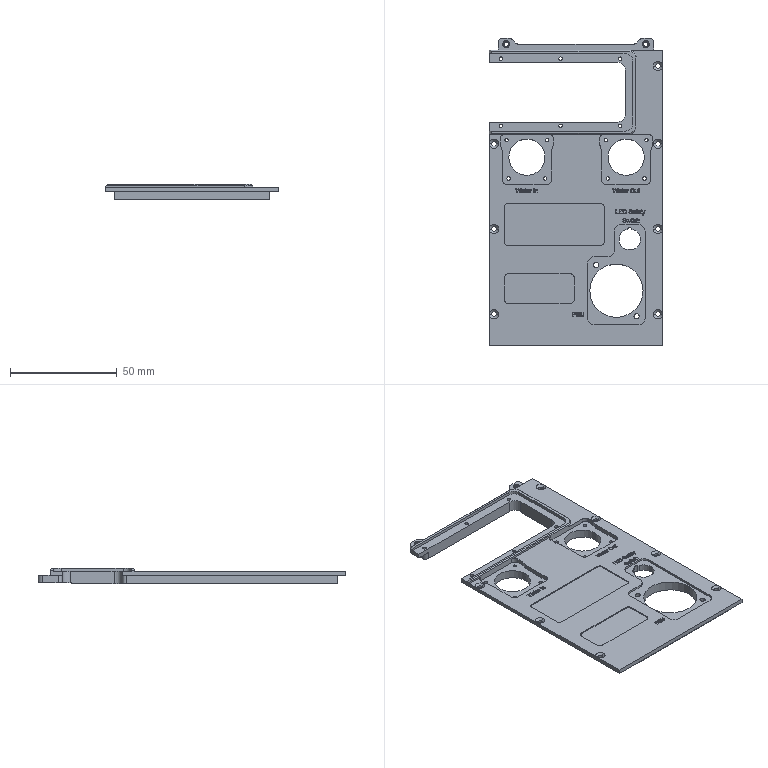NC program | NX | posted with a generic post | part box 81.5 x 144.28 x 7.5 mm
Lines 4777 to 5812 of 9048:
(PLANAR_MILL_COPY_COPY_2_COPY_2_COPY , TOOL : D4精光)
N9492 T02 M6
N9494 G54
N9496 G17 G0 G90 X63.193 Y-40.5 S6000 M3
N9498 G43 Z50. H2
N9500 Z-1.
N9502 G94 G1 Z-4. F700.
N9504 X62.84 Y-38.5
N9506 G2 X58.843 Y-34.653 R4.
N9508 G3 X57.709 Y-33.5 R1.059
N9510 G1 X35.971
N9512 G3 X34.837 Y-34.653 R1.059
N9514 G2 X30.84 Y-38.5 R4.
N9516 G1 X30.487 Y-40.5
N9518 Z-1.
N9520 G0 Z50.
(PLANAR_MILL_COPY_COPY_1_COPY_COPY_COPY_1_COPY_COPY_1_COPY_COPY_1_COPY_COPY , T)
N9522 X-19.992 Y23.358 S4500
N9524 Z-1.
N9526 G1 X-19.908 Y23.436 Z-1.002 F800.
N9528 X-19.709 Y23.808 Z-1.009
N9530 Y24.552 Z-1.022
N9532 X-19.62 Y24.893 Z-1.028
N9534 X-19.449 Y25.2 Z-1.035
N9536 X-19.62 Y25.507 Z-1.041
N9538 X-19.709 Y25.848 Z-1.047
N9540 Y26.592 Z-1.06
N9542 X-19.908 Y26.964 Z-1.067
N9544 X-20.779 Y27.756 Z-1.088
N9546 X-21.888 Y28.15 Z-1.108
N9548 X-22.732 Z-1.123
N9550 X-23.84 Y27.757 Z-1.144
N9552 X-24.71 Y26.967 Z-1.164
N9554 X-24.909 Y26.595 Z-1.172
N9556 Y23.805 Z-1.22
N9558 X-24.71 Y23.433 Z-1.228
N9560 X-23.896 Y22.677 Z-1.247
N9562 X-22.863 Y22.272 Z-1.266
N9564 X-21.753 Z-1.286
N9566 X-20.72 Y22.679 Z-1.305
N9568 X-19.908 Y23.436 Z-1.324
N9570 X-19.709 Y23.808 Z-1.332
N9572 Y24.552 Z-1.345
N9574 X-19.62 Y24.893 Z-1.351
N9576 X-19.449 Y25.2 Z-1.357
N9578 X-19.62 Y25.507 Z-1.363
N9580 X-19.709 Y25.848 Z-1.369
N9582 Y26.592 Z-1.382
N9584 X-19.908 Y26.964 Z-1.39
N9586 X-20.779 Y27.756 Z-1.41
N9588 X-21.888 Y28.15 Z-1.431
N9590 X-22.732 Z-1.446
N9592 X-23.84 Y27.757 Z-1.466
N9594 X-24.71 Y26.967 Z-1.487
N9596 X-24.909 Y26.595 Z-1.494
N9598 Y23.805 Z-1.543
N9600 X-24.71 Y23.433 Z-1.55
N9602 X-23.896 Y22.677 Z-1.569
N9604 X-22.863 Y22.272 Z-1.589
N9606 X-21.753 Z-1.608
N9608 X-20.72 Y22.679 Z-1.628
N9610 X-19.908 Y23.436 Z-1.647
N9612 X-19.709 Y23.808 Z-1.654
N9614 Y24.552 Z-1.667
N9616 X-19.62 Y24.893 Z-1.673
N9618 X-19.449 Y25.2 Z-1.68
N9620 X-19.62 Y25.507 Z-1.686
N9622 X-19.709 Y25.848 Z-1.692
N9624 Y26.592 Z-1.705
N9626 X-19.908 Y26.964 Z-1.712
N9628 X-20.779 Y27.756 Z-1.733
N9630 X-21.888 Y28.15 Z-1.753
N9632 X-22.732 Z-1.768
N9634 X-23.84 Y27.757 Z-1.789
N9636 X-24.71 Y26.967 Z-1.809
N9638 X-24.909 Y26.595 Z-1.816
N9640 Y23.805 Z-1.865
N9642 X-24.71 Y23.433 Z-1.872
N9644 X-23.896 Y22.677 Z-1.892
N9646 X-22.863 Y22.272 Z-1.911
N9648 X-21.753 Z-1.931
N9650 X-20.72 Y22.679 Z-1.95
N9652 X-19.908 Y23.436 Z-1.969
N9654 X-19.709 Y23.808 Z-1.977
N9656 Y24.552 Z-1.99
N9658 X-19.62 Y24.893 Z-1.996
N9660 X-19.449 Y25.2 Z-2.002
N9662 X-19.62 Y25.507 Z-2.008
N9664 X-19.709 Y25.848 Z-2.014
N9666 Y26.592 Z-2.027
N9668 X-19.908 Y26.964 Z-2.035
N9670 X-20.779 Y27.756 Z-2.055
N9672 X-21.888 Y28.15 Z-2.076
N9674 X-22.732 Z-2.09
N9676 X-23.84 Y27.757 Z-2.111
N9678 X-24.71 Y26.967 Z-2.131
N9680 X-24.909 Y26.595 Z-2.139
N9682 Y23.805 Z-2.188
N9684 X-24.71 Y23.433 Z-2.195
N9686 X-23.896 Y22.677 Z-2.214
N9688 X-22.863 Y22.272 Z-2.234
N9690 X-21.753 Z-2.253
N9692 X-20.72 Y22.679 Z-2.272
N9694 X-19.908 Y23.436 Z-2.292
N9696 X-19.709 Y23.808 Z-2.299
N9698 Y24.552 Z-2.312
N9700 X-19.62 Y24.893 Z-2.318
N9702 X-19.449 Y25.2 Z-2.324
N9704 X-19.62 Y25.507 Z-2.331
N9706 X-19.709 Y25.848 Z-2.337
N9708 Y26.592 Z-2.35
N9710 X-19.908 Y26.964 Z-2.357
N9712 X-20.779 Y27.756 Z-2.378
N9714 X-21.888 Y28.15 Z-2.398
N9716 X-22.732 Z-2.413
N9718 X-23.84 Y27.757 Z-2.433
N9720 X-24.71 Y26.967 Z-2.454
N9722 X-24.909 Y26.595 Z-2.461
N9724 Y23.805 Z-2.51
N9726 X-24.71 Y23.433 Z-2.517
N9728 X-23.896 Y22.677 Z-2.537
N9730 X-22.863 Y22.272 Z-2.556
N9732 X-21.753 Z-2.576
N9734 X-20.72 Y22.679 Z-2.595
N9736 X-19.908 Y23.436 Z-2.614
N9738 X-19.709 Y23.808 Z-2.622
N9740 Y24.552 Z-2.635
N9742 X-19.62 Y24.893 Z-2.641
N9744 X-19.449 Y25.2 Z-2.647
N9746 X-19.62 Y25.507 Z-2.653
N9748 X-19.709 Y25.848 Z-2.659
N9750 Y26.592 Z-2.672
N9752 X-19.908 Y26.964 Z-2.68
N9754 X-20.779 Y27.756 Z-2.7
N9756 X-21.888 Y28.15 Z-2.721
N9758 X-22.732 Z-2.735
N9760 X-23.84 Y27.757 Z-2.756
N9762 X-24.71 Y26.967 Z-2.776
N9764 X-24.909 Y26.595 Z-2.784
N9766 Y23.805 Z-2.832
N9768 X-24.71 Y23.433 Z-2.84
N9770 X-23.896 Y22.677 Z-2.859
N9772 X-22.863 Y22.272 Z-2.879
N9774 X-21.753 Z-2.898
N9776 X-20.72 Y22.679 Z-2.917
N9778 X-19.908 Y23.436 Z-2.937
N9780 X-19.709 Y23.808 Z-2.944
N9782 Y24.552 Z-2.957
N9784 X-19.62 Y24.893 Z-2.963
N9786 X-19.449 Y25.2 Z-2.969
N9788 X-19.62 Y25.507 Z-2.976
N9790 X-19.709 Y25.848 Z-2.982
N9792 Y26.592 Z-2.995
N9794 X-19.908 Y26.964 Z-3.002
N9796 X-20.779 Y27.756 Z-3.023
N9798 X-21.888 Y28.15 Z-3.043
N9800 X-22.732 Z-3.058
N9802 X-23.84 Y27.757 Z-3.078
N9804 X-24.71 Y26.967 Z-3.099
N9806 X-24.909 Y26.595 Z-3.106
N9808 Y23.805 Z-3.155
N9810 X-24.71 Y23.433 Z-3.162
N9812 X-23.896 Y22.677 Z-3.182
N9814 X-22.863 Y22.272 Z-3.201
N9816 X-21.753 Z-3.22
N9818 X-20.72 Y22.679 Z-3.24
N9820 X-19.908 Y23.436 Z-3.259
N9822 X-19.709 Y23.808 Z-3.267
N9824 Y24.552 Z-3.28
N9826 X-19.62 Y24.893 Z-3.286
N9828 X-19.449 Y25.2 Z-3.292
N9830 X-19.62 Y25.507 Z-3.298
N9832 X-19.709 Y25.848 Z-3.304
N9834 Y26.592 Z-3.317
N9836 X-19.908 Y26.964 Z-3.324
N9838 X-20.779 Y27.756 Z-3.345
N9840 X-21.888 Y28.15 Z-3.366
N9842 X-22.732 Z-3.38
N9844 X-23.84 Y27.757 Z-3.401
N9846 X-24.71 Y26.967 Z-3.421
N9848 X-24.909 Y26.595 Z-3.429
N9850 Y23.805 Z-3.477
N9852 X-24.71 Y23.433 Z-3.485
N9854 X-23.896 Y22.677 Z-3.504
N9856 X-22.863 Y22.272 Z-3.523
N9858 X-21.753 Z-3.543
N9860 X-20.72 Y22.679 Z-3.562
N9862 X-19.908 Y23.436 Z-3.582
N9864 X-19.709 Y23.808 Z-3.589
N9866 Y24.552 Z-3.602
N9868 X-19.62 Y24.893 Z-3.608
N9870 X-19.449 Y25.2 Z-3.614
N9872 X-19.62 Y25.507 Z-3.62
N9874 X-19.709 Y25.848 Z-3.627
N9876 Y26.592 Z-3.64
N9878 X-19.908 Y26.964 Z-3.647
N9880 X-20.779 Y27.756 Z-3.667
N9882 X-21.888 Y28.15 Z-3.688
N9884 X-22.732 Z-3.703
N9886 X-23.84 Y27.757 Z-3.723
N9888 X-24.71 Y26.967 Z-3.744
N9890 X-24.909 Y26.595 Z-3.751
N9892 Y23.805 Z-3.8
N9894 X-24.71 Y23.433 Z-3.807
N9896 X-23.896 Y22.677 Z-3.827
N9898 X-22.863 Y22.272 Z-3.846
N9900 X-21.753 Z-3.865
N9902 X-20.72 Y22.679 Z-3.885
N9904 X-19.908 Y23.436 Z-3.904
N9906 X-19.709 Y23.808 Z-3.911
N9908 Y24.552 Z-3.924
N9910 X-19.62 Y24.893 Z-3.931
N9912 X-19.449 Y25.2 Z-3.937
N9914 X-19.62 Y25.507 Z-3.943
N9916 X-19.709 Y25.848 Z-3.949
N9918 Y26.592 Z-3.962
N9920 X-19.908 Y26.964 Z-3.969
N9922 X-20.779 Y27.756 Z-3.99
N9924 X-21.888 Y28.15 Z-4.01
N9926 X-22.732 Z-4.025
N9928 X-23.84 Y27.757 Z-4.046
N9930 X-24.71 Y26.967 Z-4.066
N9932 X-24.909 Y26.595 Z-4.074
N9934 Y23.805 Z-4.122
N9936 X-24.71 Y23.433 Z-4.13
N9938 X-23.896 Y22.677 Z-4.149
N9940 X-22.863 Y22.272 Z-4.168
N9942 X-21.753 Z-4.188
N9944 X-20.72 Y22.679 Z-4.207
N9946 X-19.908 Y23.436 Z-4.227
N9948 X-19.709 Y23.808 Z-4.234
N9950 Y24.552 Z-4.247
N9952 X-19.62 Y24.893 Z-4.253
N9954 X-19.449 Y25.2 Z-4.259
N9956 X-19.62 Y25.507 Z-4.265
N9958 X-19.709 Y25.848 Z-4.271
N9960 Y26.592 Z-4.284
N9962 X-19.908 Y26.964 Z-4.292
N9964 X-20.779 Y27.756 Z-4.312
N9966 X-21.888 Y28.15 Z-4.333
N9968 X-22.732 Z-4.348
N9970 X-23.84 Y27.757 Z-4.368
N9972 X-24.71 Y26.967 Z-4.389
N9974 X-24.909 Y26.595 Z-4.396
N9976 Y23.805 Z-4.445
N9978 X-24.71 Y23.433 Z-4.452
N9980 X-23.896 Y22.677 Z-4.471
N9982 X-22.863 Y22.272 Z-4.491
N9984 X-21.753 Z-4.51
N9986 X-20.72 Y22.679 Z-4.53
N9988 X-19.908 Y23.436 Z-4.549
N9990 X-19.709 Y23.808 Z-4.556
N9992 Y24.552 Z-4.569
N9994 X-19.62 Y24.893 Z-4.575
N9996 X-19.449 Y25.2 Z-4.582
N9998 X-19.62 Y25.507 Z-4.588
N10000 X-19.709 Y25.848 Z-4.594
N10002 Y26.592 Z-4.607
N10004 X-19.908 Y26.964 Z-4.614
N10006 X-20.779 Y27.756 Z-4.635
N10008 X-21.888 Y28.15 Z-4.655
N10010 X-22.732 Z-4.67
N10012 X-23.84 Y27.757 Z-4.691
N10014 X-24.71 Y26.967 Z-4.711
N10016 X-24.909 Y26.595 Z-4.718
N10018 Y23.805 Z-4.767
N10020 X-24.71 Y23.433 Z-4.775
N10022 X-23.896 Y22.677 Z-4.794
N10024 X-22.863 Y22.272 Z-4.813
N10026 X-21.753 Z-4.833
N10028 X-20.72 Y22.679 Z-4.852
N10030 X-19.908 Y23.436 Z-4.871
N10032 X-19.709 Y23.808 Z-4.879
N10034 Y24.552 Z-4.892
N10036 X-19.62 Y24.893 Z-4.898
N10038 X-19.449 Y25.2 Z-4.904
N10040 X-19.62 Y25.507 Z-4.91
N10042 X-19.709 Y25.848 Z-4.916
N10044 Y26.592 Z-4.929
N10046 X-19.908 Y26.964 Z-4.937
N10048 X-20.779 Y27.756 Z-4.957
N10050 X-21.888 Y28.15 Z-4.978
N10052 X-22.732 Z-4.993
N10054 X-23.84 Y27.757 Z-5.013
N10056 X-24.71 Y26.967 Z-5.034
N10058 X-24.909 Y26.595 Z-5.041
N10060 Y23.805 Z-5.09
N10062 X-24.71 Y23.433 Z-5.097
N10064 X-23.896 Y22.677 Z-5.116
N10066 X-22.863 Y22.272 Z-5.136
N10068 X-21.753 Z-5.155
N10070 X-20.72 Y22.679 Z-5.175
N10072 X-19.908 Y23.436 Z-5.194
N10074 X-19.709 Y23.808 Z-5.201
N10076 Y24.552 Z-5.214
N10078 X-19.62 Y24.893 Z-5.22
N10080 X-19.449 Y25.2 Z-5.227
N10082 X-19.62 Y25.507 Z-5.233
N10084 X-19.709 Y25.848 Z-5.239
N10086 Y26.592 Z-5.252
N10088 X-19.908 Y26.964 Z-5.259
N10090 X-20.779 Y27.756 Z-5.28
N10092 X-21.888 Y28.15 Z-5.3
N10094 X-22.732 Z-5.315
N10096 X-23.84 Y27.757 Z-5.336
N10098 X-24.71 Y26.967 Z-5.356
N10100 X-24.909 Y26.595 Z-5.363
N10102 Y23.805 Z-5.412
N10104 X-24.71 Y23.433 Z-5.419
N10106 X-23.896 Y22.677 Z-5.439
N10108 X-22.863 Y22.272 Z-5.458
N10110 X-21.753 Z-5.478
N10112 X-20.72 Y22.679 Z-5.497
N10114 X-19.908 Y23.436 Z-5.516
N10116 X-19.709 Y23.808 Z-5.524
N10118 Y24.552 Z-5.537
N10120 X-19.62 Y24.893 Z-5.543
N10122 X-19.449 Y25.2 Z-5.549
N10124 X-19.62 Y25.507 Z-5.555
N10126 X-19.709 Y25.848 Z-5.561
N10128 Y26.592 Z-5.574
N10130 X-19.908 Y26.964 Z-5.582
N10132 X-20.779 Y27.756 Z-5.602
N10134 X-21.888 Y28.15 Z-5.623
N10136 X-22.732 Z-5.637
N10138 X-23.84 Y27.757 Z-5.658
N10140 X-24.71 Y26.967 Z-5.678
N10142 X-24.909 Y26.595 Z-5.686
N10144 Y23.805 Z-5.735
N10146 X-24.71 Y23.433 Z-5.742
N10148 X-23.896 Y22.677 Z-5.761
N10150 X-22.863 Y22.272 Z-5.781
N10152 X-21.753 Z-5.8
N10154 X-20.72 Y22.679 Z-5.819
N10156 X-19.908 Y23.436 Z-5.839
N10158 X-19.709 Y23.808 Z-5.846
N10160 Y24.552 Z-5.859
N10162 X-19.62 Y24.893 Z-5.865
N10164 X-19.449 Y25.2 Z-5.871
N10166 X-19.62 Y25.507 Z-5.878
N10168 X-19.709 Y25.848 Z-5.884
N10170 Y26.592 Z-5.897
N10172 X-19.908 Y26.964 Z-5.904
N10174 X-20.779 Y27.756 Z-5.925
N10176 X-21.888 Y28.15 Z-5.945
N10178 X-22.732 Z-5.96
N10180 X-23.84 Y27.757 Z-5.98
N10182 X-24.71 Y26.967 Z-6.001
N10184 X-24.909 Y26.595 Z-6.008
N10186 Y23.805 Z-6.057
N10188 X-24.71 Y23.433 Z-6.064
N10190 X-23.896 Y22.677 Z-6.084
N10192 X-22.863 Y22.272 Z-6.103
N10194 X-21.753 Z-6.122
N10196 X-20.72 Y22.679 Z-6.142
N10198 X-19.908 Y23.436 Z-6.161
N10200 X-19.709 Y23.808 Z-6.169
N10202 Y24.552 Z-6.182
N10204 X-19.62 Y24.893 Z-6.188
N10206 X-19.449 Y25.2 Z-6.194
N10208 X-19.62 Y25.507 Z-6.2
N10210 X-19.709 Y25.848 Z-6.206
N10212 Y26.592 Z-6.219
N10214 X-19.908 Y26.964 Z-6.227
N10216 X-20.779 Y27.756 Z-6.247
N10218 X-21.888 Y28.15 Z-6.268
N10220 X-22.732 Z-6.282
N10222 X-23.84 Y27.757 Z-6.303
N10224 X-24.71 Y26.967 Z-6.323
N10226 X-24.909 Y26.595 Z-6.331
N10228 Y23.805 Z-6.379
N10230 X-24.71 Y23.433 Z-6.387
N10232 X-23.896 Y22.677 Z-6.406
N10234 X-22.863 Y22.272 Z-6.426
N10236 X-21.753 Z-6.445
N10238 X-20.72 Y22.679 Z-6.464
N10240 X-19.908 Y23.436 Z-6.484
N10242 X-19.709 Y23.808 Z-6.491
N10244 Y24.552 Z-6.504
N10246 X-19.62 Y24.893 Z-6.51
N10248 X-19.449 Y25.2 Z-6.516
N10250 X-19.62 Y25.507 Z-6.522
N10252 X-19.709 Y25.848 Z-6.529
N10254 Y26.592 Z-6.542
N10256 X-19.908 Y26.964 Z-6.549
N10258 X-20.779 Y27.756 Z-6.57
N10260 X-21.888 Y28.15 Z-6.59
N10262 X-22.732 Z-6.605
N10264 X-23.84 Y27.757 Z-6.625
N10266 X-24.71 Y26.967 Z-6.646
N10268 X-24.909 Y26.595 Z-6.653
N10270 Y23.805 Z-6.702
N10272 X-24.71 Y23.433 Z-6.709
N10274 X-23.896 Y22.677 Z-6.729
N10276 X-22.863 Y22.272 Z-6.748
N10278 X-21.753 Z-6.767
N10280 X-20.72 Y22.679 Z-6.787
N10282 X-19.908 Y23.436 Z-6.806
N10284 X-19.709 Y23.808 Z-6.814
N10286 Y24.552 Z-6.826
N10288 X-19.62 Y24.893 Z-6.833
N10290 X-19.449 Y25.2 Z-6.839
N10292 X-19.62 Y25.507 Z-6.845
N10294 X-19.709 Y25.848 Z-6.851
N10296 Y26.592 Z-6.864
N10298 X-19.908 Y26.964 Z-6.871
N10300 X-20.779 Y27.756 Z-6.892
N10302 X-21.888 Y28.15 Z-6.913
N10304 X-22.732 Z-6.927
N10306 X-23.84 Y27.757 Z-6.948
N10308 X-24.71 Y26.967 Z-6.968
N10310 X-24.909 Y26.595 Z-6.976
N10312 Y25.2 Z-7.
N10314 Y23.805
N10316 G3 X-19.709 Y23.808 R2.95
N10318 G1 Y24.2
N10320 G2 X-19.449 Y25.2 R2.05
N10322 X-19.709 Y26.2 R2.05
N10324 G1 Y26.592
N10326 G3 X-24.909 Y26.595 R2.95
N10328 G1 Y25.2
N10330 Z-6.
N10332 G0 Z50.
(CAVITY_MILL_COPY , TOOL : D4精光)
N10334 X-63.162 Y33.
N10336 Z3.1
N10338 Z0.1
N10340 G1 Z-0.4
N10342 G3 X-63.562 Y33.4 R0.4
N10344 G1 X-64.21
N10346 Y32.752
N10348 G3 X-63.81 Y32.352 R0.4
N10350 G1 Z0.1
N10352 G0 Z3.
N10354 Y7.648
N10356 Z0.1
N10358 G1 Z-0.4
N10360 G3 X-64.21 Y7.248 R0.4
N10362 G1 Y6.6
N10364 X-63.562
N10366 G3 X-63.162 Y7. R0.4
N10368 G1 Z0.1
N10370 G0 Z3.1
N10372 Y0.
N10374 Z0.1
N10376 G1 Z-0.4
N10378 G3 X-63.562 Y0.4 R0.4
N10380 G1 X-64.21
N10382 Y-0.248
N10384 G3 X-63.81 Y-0.648 R0.4
N10386 G1 Z0.1
N10388 G0 Z0.5
N10390 X-63.162 Y0.
N10392 Z-0.65
N10394 G1 Z-1.15
N10396 G3 X-63.562 Y0.4 R0.4
N10398 G1 X-64.21
N10400 Y-0.248
N10402 G3 X-63.81 Y-0.648 R0.4
N10404 G1 Z-0.65
N10406 G0 Z0.1
N10408 X-63.162 Y0.
N10410 Z-1.4
N10412 G1 Z-1.9
N10414 G3 X-63.562 Y0.4 R0.4
N10416 G1 X-64.21
N10418 Y-0.248
N10420 G3 X-63.81 Y-0.648 R0.4
N10422 G1 Z-1.4
N10424 G0 Z-0.65
N10426 X-63.162 Y0.
N10428 Z-1.9
N10430 G1 Z-2.4
N10432 G3 X-63.562 Y0.4 R0.4
N10434 G1 X-64.21
N10436 Y-0.248
N10438 G3 X-63.81 Y-0.648 R0.4
N10440 G1 Z-1.9
N10442 G0 Z-1.4
N10444 X-63.162 Y0.
N10446 Z-2.4
N10448 G1 Z-2.9
N10450 G3 X-63.562 Y0.4 R0.4
N10452 G1 X-64.21
N10454 Y-0.248
N10456 G3 X-63.81 Y-0.648 R0.4
N10458 G1 Z-2.4
N10460 G0 Z3.
N10462 Y-31.352
N10464 Z0.1
N10466 G1 Z-0.4
N10468 G3 X-64.21 Y-31.752 R0.4
N10470 G1 Y-32.4
N10472 X-63.562
N10474 G3 X-63.162 Y-32. R0.4
N10476 G1 Z0.1
N10478 G0 Z0.5
N10480 X-63.81 Y-31.352
N10482 Z-0.65
N10484 G1 Z-1.15
N10486 G3 X-64.21 Y-31.752 R0.4
N10488 G1 Y-32.4
N10490 X-63.562
N10492 G3 X-63.162 Y-32. R0.4
N10494 G1 Z-0.65
N10496 G0 Z0.1
N10498 X-63.81 Y-31.352
N10500 Z-1.4
N10502 G1 Z-1.9
N10504 G3 X-64.21 Y-31.752 R0.4
N10506 G1 Y-32.4
N10508 X-63.562
N10510 G3 X-63.162 Y-32. R0.4
N10512 G1 Z-1.4
N10514 G0 Z-0.65
N10516 X-63.81 Y-31.352
N10518 Z-1.9
N10520 G1 Z-2.4
N10522 G3 X-64.21 Y-31.752 R0.4
N10524 G1 Y-32.4
N10526 X-63.562
N10528 G3 X-63.162 Y-32. R0.4
N10530 G1 Z-1.9
N10532 G0 Z-1.4
N10534 X-63.81 Y-31.352
N10536 Z-2.4
N10538 G1 Z-2.9
N10540 G3 X-64.21 Y-31.752 R0.4
N10542 G1 Y-32.4
N10544 X-63.562
N10546 G3 X-63.162 Y-32. R0.4
N10548 G1 Z-2.4
N10550 G0 Z3.
N10552 X-33.458
N10554 Z0.1
N10556 G1 Z-0.4
N10558 G3 X-33.058 Y-32.4 R0.4
N10560 G1 X-32.41
N10562 Y-31.752
N10564 G3 X-32.81 Y-31.352 R0.4
N10566 G1 Z0.1
N10568 G0 Z0.5
N10570 X-33.458 Y-32.
N10572 Z-0.65
N10574 G1 Z-1.15
N10576 G3 X-33.058 Y-32.4 R0.4
N10578 G1 X-32.41
N10580 Y-31.752
N10582 G3 X-32.81 Y-31.352 R0.4
N10584 G1 Z-0.65
N10586 G0 Z0.1
N10588 X-33.458 Y-32.
N10590 Z-1.4
N10592 G1 Z-1.9
N10594 G3 X-33.058 Y-32.4 R0.4
N10596 G1 X-32.41
N10598 Y-31.752
N10600 G3 X-32.81 Y-31.352 R0.4
N10602 G1 Z-1.4
N10604 G0 Z-0.65
N10606 X-33.458 Y-32.
N10608 Z-1.9
N10610 G1 Z-2.4
N10612 G3 X-33.058 Y-32.4 R0.4
N10614 G1 X-32.41
N10616 Y-31.752
N10618 G3 X-32.81 Y-31.352 R0.4
N10620 G1 Z-1.9
N10622 G0 Z-1.4
N10624 X-33.458 Y-32.
N10626 Z-2.4
N10628 G1 Z-2.9
N10630 G3 X-33.058 Y-32.4 R0.4
N10632 G1 X-32.41
N10634 Y-31.752
N10636 G3 X-32.81 Y-31.352 R0.4
N10638 G1 Z-2.4
N10640 G0 Z3.1
N10642 X-25.81
N10644 Z0.1
N10646 G1 Z-0.4
N10648 G3 X-26.21 Y-31.752 R0.4
N10650 G1 Y-32.4
N10652 X-25.562
N10654 G3 X-25.162 Y-32. R0.4
N10656 G1 Z0.1
N10658 G0 Z0.5
N10660 X-25.81 Y-31.352
N10662 Z-0.65
N10664 G1 Z-1.15
N10666 G3 X-26.21 Y-31.752 R0.4
N10668 G1 Y-32.4
N10670 X-25.562
N10672 G3 X-25.162 Y-32. R0.4
N10674 G1 Z-0.65
N10676 G0 Z0.1
N10678 X-25.81 Y-31.352
N10680 Z-1.4
N10682 G1 Z-1.9
N10684 G3 X-26.21 Y-31.752 R0.4
N10686 G1 Y-32.4
N10688 X-25.562
N10690 G3 X-25.162 Y-32. R0.4
N10692 G1 Z-1.4
N10694 G0 Z-0.65
N10696 X-25.81 Y-31.352
N10698 Z-1.9
N10700 G1 Z-2.4
N10702 G3 X-26.21 Y-31.752 R0.4
N10704 G1 Y-32.4
N10706 X-25.562
N10708 G3 X-25.162 Y-32. R0.4
N10710 G1 Z-1.9
N10712 G0 Z-1.4
N10714 X-25.81 Y-31.352
N10716 Z-2.4
N10718 G1 Z-2.9
N10720 G3 X-26.21 Y-31.752 R0.4
N10722 G1 Y-32.4
N10724 X-25.562
N10726 G3 X-25.162 Y-32. R0.4
N10728 G1 Z-2.4
N10730 G0 Z3.
N10732 Y-16.05
N10734 Z0.1
N10736 G1 Z-0.4
N10738 G3 X-25.562 Y-15.65 R0.4
N10740 G1 X-26.21
N10742 Y-16.298
N10744 G3 X-25.81 Y-16.698 R0.4
N10746 G1 Z0.1
N10748 G0 Z0.5
N10750 X-25.162 Y-16.05
N10752 Z-0.65
N10754 G1 Z-1.15
N10756 G3 X-25.562 Y-15.65 R0.4
N10758 G1 X-26.21
N10760 Y-16.298
N10762 G3 X-25.81 Y-16.698 R0.4
N10764 G1 Z-0.65
N10766 G0 Z0.1
N10768 X-25.162 Y-16.05
N10770 Z-1.4
N10772 G1 Z-1.9
N10774 G3 X-25.562 Y-15.65 R0.4
N10776 G1 X-26.21
N10778 Y-16.298
N10780 G3 X-25.81 Y-16.698 R0.4
N10782 G1 Z-1.4
N10784 G0 Z-0.65
N10786 X-25.162 Y-16.05
N10788 Z-1.9
N10790 G1 Z-2.4
N10792 G3 X-25.562 Y-15.65 R0.4
N10794 G1 X-26.21
N10796 Y-16.298
N10798 G3 X-25.81 Y-16.698 R0.4
N10800 G1 Z-1.9
N10802 G0 Z-1.4
N10804 X-25.162 Y-16.05
N10806 Z-2.4
N10808 G1 Z-2.9
N10810 G3 X-25.562 Y-15.65 R0.4
N10812 G1 X-26.21
N10814 Y-16.298
N10816 G3 X-25.81 Y-16.698 R0.4
N10818 G1 Z-2.4
N10820 G0 Z3.1
N10822 Y-8.402
N10824 Z0.1
N10826 G1 Z-0.4
N10828 G3 X-26.21 Y-8.802 R0.4
N10830 G1 Y-9.45
N10832 X-25.562
N10834 G3 X-25.162 Y-9.05 R0.4
N10836 G1 Z0.1
N10838 G0 Z0.5
N10840 X-25.81 Y-8.402
N10842 Z-0.65
N10844 G1 Z-1.15
N10846 G3 X-26.21 Y-8.802 R0.4
N10848 G1 Y-9.45
N10850 X-25.562
N10852 G3 X-25.162 Y-9.05 R0.4
N10854 G1 Z-0.65
N10856 G0 Z0.1
N10858 X-25.81 Y-8.402
N10860 Z-1.4
N10862 G1 Z-1.9
N10864 G3 X-26.21 Y-8.802 R0.4
N10866 G1 Y-9.45
N10868 X-25.562
N10870 G3 X-25.162 Y-9.05 R0.4
N10872 G1 Z-1.4
N10874 G0 Z-0.65
N10876 X-25.81 Y-8.402
N10878 Z-1.9
N10880 G1 Z-2.4
N10882 G3 X-26.21 Y-8.802 R0.4
N10884 G1 Y-9.45
N10886 X-25.562
N10888 G3 X-25.162 Y-9.05 R0.4
N10890 G1 Z-1.9
N10892 G0 Z-1.4
N10894 X-25.81 Y-8.402
N10896 Z-2.4
N10898 G1 Z-2.9
N10900 G3 X-26.21 Y-8.802 R0.4
N10902 G1 Y-9.45
N10904 X-25.562
N10906 G3 X-25.162 Y-9.05 R0.4
N10908 G1 Z-2.4
N10910 G0 Z3.1
N10912 X-32.81 Y-0.648
N10914 Z0.1
N10916 G1 Z-0.4
N10918 G3 X-32.41 Y-0.248 R0.4
N10920 G1 Y0.4
N10922 X-33.058
N10924 G3 X-33.458 Y0. R0.4
N10926 G1 Z0.1
N10928 G0 Z0.5
N10930 X-32.81 Y-0.648
N10932 Z-0.65
N10934 G1 Z-1.15
N10936 G3 X-32.41 Y-0.248 R0.4
N10938 G1 Y0.4
N10940 X-33.058
N10942 G3 X-33.458 Y0. R0.4
N10944 G1 Z-0.65
N10946 G0 Z0.1
N10948 X-32.81 Y-0.648
N10950 Z-1.4
N10952 G1 Z-1.9
N10954 G3 X-32.41 Y-0.248 R0.4
N10956 G1 Y0.4
N10958 X-33.058
N10960 G3 X-33.458 Y0. R0.4
N10962 G1 Z-1.4
N10964 G0 Z-0.65
N10966 X-32.81 Y-0.648
N10968 Z-1.9
N10970 G1 Z-2.4
N10972 G3 X-32.41 Y-0.248 R0.4
N10974 G1 Y0.4
N10976 X-33.058
N10978 G3 X-33.458 Y0. R0.4
N10980 G1 Z-1.9
N10982 G0 Z-1.4
N10984 X-32.81 Y-0.648
N10986 Z-2.4
N10988 G1 Z-2.9
N10990 G3 X-32.41 Y-0.248 R0.4
N10992 G1 Y0.4
N10994 X-33.058
N10996 G3 X-33.458 Y0. R0.4
N10998 G1 Z-2.4
N11000 G0 Z3.1
N11002 Y7.
N11004 Z0.1
N11006 G1 Z-0.4
N11008 G3 X-33.058 Y6.6 R0.4
N11010 G1 X-32.41
N11012 Y7.248
N11014 G3 X-32.81 Y7.648 R0.4
N11016 G1 Z0.1
N11018 G0 Z3.1
N11020 X-25.162 Y9.35
N11022 Z0.1
N11024 G1 Z-0.4
N11026 G3 X-25.562 Y9.75 R0.4
N11028 G1 X-26.21
N11030 Y9.102
N11032 G3 X-25.81 Y8.702 R0.4
N11034 G1 Z0.1
N11036 G0 Z0.5
N11038 X-25.162 Y9.35
N11040 Z-0.65
N11042 G1 Z-1.15
N11044 G3 X-25.562 Y9.75 R0.4
N11046 G1 X-26.21
N11048 Y9.102
N11050 G3 X-25.81 Y8.702 R0.4
N11052 G1 Z-0.65
N11054 G0 Z0.1
N11056 X-25.162 Y9.35
N11058 Z-1.4
N11060 G1 Z-1.9
N11062 G3 X-25.562 Y9.75 R0.4
N11064 G1 X-26.21
N11066 Y9.102
N11068 G3 X-25.81 Y8.702 R0.4
N11070 G1 Z-1.4
N11072 G0 Z-0.65
N11074 X-25.162 Y9.35
N11076 Z-1.9
N11078 G1 Z-2.4
N11080 G3 X-25.562 Y9.75 R0.4
N11082 G1 X-26.21
N11084 Y9.102
N11086 G3 X-25.81 Y8.702 R0.4
N11088 G1 Z-1.9
N11090 G0 Z-1.4
N11092 X-25.162 Y9.35
N11094 Z-2.4
N11096 G1 Z-2.9
N11098 G3 X-25.562 Y9.75 R0.4
N11100 G1 X-26.21
N11102 Y9.102
N11104 G3 X-25.81 Y8.702 R0.4
N11106 G1 Z-2.4
N11108 G0 Z3.1
N11110 X-27.81 Y17.998
N11112 Z-0.65
N11114 G1 Z-1.15
N11116 G3 X-28.21 Y17.598 R0.4
N11118 G1 Y16.95
N11120 X-27.562
N11122 G3 X-27.162 Y17.35 R0.4
N11124 G1 Z-0.65
N11126 G0 Z0.1
N11128 X-27.81 Y17.998
N11130 Z-1.4
N11132 G1 Z-1.9
N11134 G3 X-28.21 Y17.598 R0.4
N11136 G1 Y16.95
N11138 X-27.562
N11140 G3 X-27.162 Y17.35 R0.4
N11142 G1 Z-1.4
N11144 G0 Z3.
N11146 Y33.
N11148 Z-0.65
N11150 G1 Z-1.15
N11152 G3 X-27.562 Y33.4 R0.4
N11154 G1 X-28.21
N11156 Y32.752
N11158 G3 X-27.81 Y32.352 R0.4
N11160 G1 Z-0.65
N11162 G0 Z0.1
N11164 X-27.162 Y33.
N11166 Z-1.4
N11168 G1 Z-1.9
N11170 G3 X-27.562 Y33.4 R0.4
N11172 G1 X-28.21
N11174 Y32.752
N11176 G3 X-27.81 Y32.352 R0.4
N11178 G1 Z-1.4
N11180 G0 Z3.
N11182 X-20.043 Y24.954
N11184 Z-1.9
N11186 G1 Z-2.4
N11188 G3 X-19.535 Y25.144 R0.4
N11190 G1 X-19.506 Y25.2
N11192 X-19.535 Y25.256
N11194 G3 X-20.043 Y25.446 R0.4
N11196 G1 Z-1.9
N11198 G0 Z-1.4
N11200 Y24.954
N11202 Z-2.4
N11204 G1 Z-2.9
N11206 G3 X-19.535 Y25.144 R0.4
N11208 G1 X-19.506 Y25.2
N11210 X-19.535 Y25.256
N11212 G3 X-20.043 Y25.446 R0.4
N11214 G1 Z-2.4
N11216 G0 Z-1.9
N11218 Y24.954
N11220 Z-2.9
N11222 G1 Z-3.4
N11224 G3 X-19.535 Y25.144 R0.4
N11226 G1 X-19.506 Y25.2
N11228 X-19.535 Y25.256
N11230 G3 X-20.043 Y25.446 R0.4
N11232 G1 Z-2.9
N11234 G0 Z-2.4
N11236 Y24.954
N11238 Z-3.4
N11240 G1 Z-3.9
N11242 G3 X-19.535 Y25.144 R0.4
N11244 G1 X-19.506 Y25.2
N11246 X-19.535 Y25.256
N11248 G3 X-20.043 Y25.446 R0.4
N11250 G1 Z-3.4
N11252 G0 Z-2.9
N11254 Y24.954
N11256 Z-4.05
N11258 G1 Z-4.55
N11260 G3 X-19.535 Y25.144 R0.4
N11262 G1 X-19.506 Y25.2
N11264 X-19.535 Y25.256
N11266 G3 X-20.043 Y25.446 R0.4
N11268 G1 Z-4.05
N11270 G0 Z-3.4
N11272 X-20.049 Y24.933
N11274 Z-4.7
N11276 G1 Z-5.2
N11278 G3 X-19.543 Y25.128 R0.4
N11280 G1 X-19.506 Y25.2
N11282 X-19.545 Y25.276
N11284 G3 X-20.051 Y25.473 R0.4
N11286 G1 Z-4.7
N11288 G0 Z-4.05
N11290 X-20.049 Y24.933
N11292 Z-5.35
N11294 G1 Z-5.85
N11296 G3 X-19.543 Y25.128 R0.4
N11298 G1 X-19.506 Y25.2
N11300 X-19.545 Y25.276
N11302 G3 X-20.051 Y25.473 R0.4
N11304 G1 Z-5.35
N11306 G0 Z-4.7
N11308 X-20.049 Y24.933
N11310 Z-6.
N11312 G1 Z-6.5
N11314 G3 X-19.543 Y25.128 R0.4
N11316 G1 X-19.506 Y25.2
N11318 X-19.545 Y25.276
N11320 G3 X-20.051 Y25.473 R0.4
N11322 G1 Z-6.
N11324 G0 Z3.
N11326 X0.992 Y17.35
N11328 Z0.1
N11330 G1 Z-0.4
N11332 G3 X1.392 Y16.95 R0.4
N11334 G1 X2.04
N11336 Y17.598
N11338 G3 X1.64 Y17.998 R0.4
N11340 G1 Z0.1
N11342 G0 Z0.5
N11344 X0.992 Y17.35
N11346 Z-0.65
N11348 G1 Z-1.15
N11350 G3 X1.392 Y16.95 R0.4
N11352 G1 X2.04
N11354 Y17.598
N11356 G3 X1.64 Y17.998 R0.4
N11358 G1 Z-0.65
N11360 G0 Z0.1
N11362 X0.992 Y17.35
N11364 Z-1.4
N11366 G1 Z-1.9
N11368 G3 X1.392 Y16.95 R0.4
N11370 G1 X2.04
N11372 Y17.598
N11374 G3 X1.64 Y17.998 R0.4
N11376 G1 Z-1.4
N11378 G0 Z3.
N11380 Y32.352
N11382 Z0.1
N11384 G1 Z-0.4
N11386 G3 X2.04 Y32.752 R0.4
N11388 G1 Y33.4
N11390 X1.392
N11392 G3 X0.992 Y33. R0.4
N11394 G1 Z0.1
N11396 G0 Z0.5
N11398 X1.64 Y32.352
N11400 Z-0.65
N11402 G1 Z-1.15
N11404 G3 X2.04 Y32.752 R0.4
N11406 G1 Y33.4
N11408 X1.392
N11410 G3 X0.992 Y33. R0.4
N11412 G1 Z-0.65
N11414 G0 Z0.1
N11416 X1.64 Y32.352
N11418 Z-1.4
N11420 G1 Z-1.9
N11422 G3 X2.04 Y32.752 R0.4
N11424 G1 Y33.4
N11426 X1.392
N11428 G3 X0.992 Y33. R0.4
N11430 G1 Z-1.4
N11432 G0 Z3.1
N11434 X29.688 Y32.
N11436 Z0.1
N11438 G1 Z-0.4
N11440 G3 X29.288 Y32.4 R0.4
N11442 G1 X28.64
N11444 Y31.752
N11446 G3 X29.04 Y31.352 R0.4
N11448 G1 Z0.1
N11450 G0 Z0.5
N11452 X29.688 Y32.
N11454 Z-0.65
N11456 G1 Z-1.15
N11458 G3 X29.288 Y32.4 R0.4
N11460 G1 X28.64
N11462 Y31.752
N11464 G3 X29.04 Y31.352 R0.4
N11466 G1 Z-0.65
N11468 G0 Z0.1
N11470 X29.688 Y32.
N11472 Z-1.4
N11474 G1 Z-1.9
N11476 G3 X29.288 Y32.4 R0.4
N11478 G1 X28.64
N11480 Y31.752
N11482 G3 X29.04 Y31.352 R0.4
N11484 G1 Z-1.4
N11486 G0 Z-0.65
N11488 X29.688 Y32.
N11490 Z-1.9
N11492 G1 Z-2.4
N11494 G3 X29.288 Y32.4 R0.4
N11496 G1 X28.64
N11498 Y31.752
N11500 G3 X29.04 Y31.352 R0.4
N11502 G1 Z-1.9
N11504 G0 Z-1.4
N11506 X29.688 Y32.
N11508 Z-2.4
N11510 G1 Z-2.9
N11512 G3 X29.288 Y32.4 R0.4
N11514 G1 X28.64
N11516 Y31.752
N11518 G3 X29.04 Y31.352 R0.4
N11520 G1 Z-2.4
N11522 G0 Z3.
N11524 Y28.398
N11526 Z0.1
N11528 G1 Z-0.4
N11530 G3 X28.64 Y27.998 R0.4
N11532 G1 Y27.35
N11534 X29.288
N11536 G3 X29.688 Y27.75 R0.4
N11538 G1 Z0.1
N11540 G0 Z0.5
N11542 X29.04 Y28.398
N11544 Z-0.65